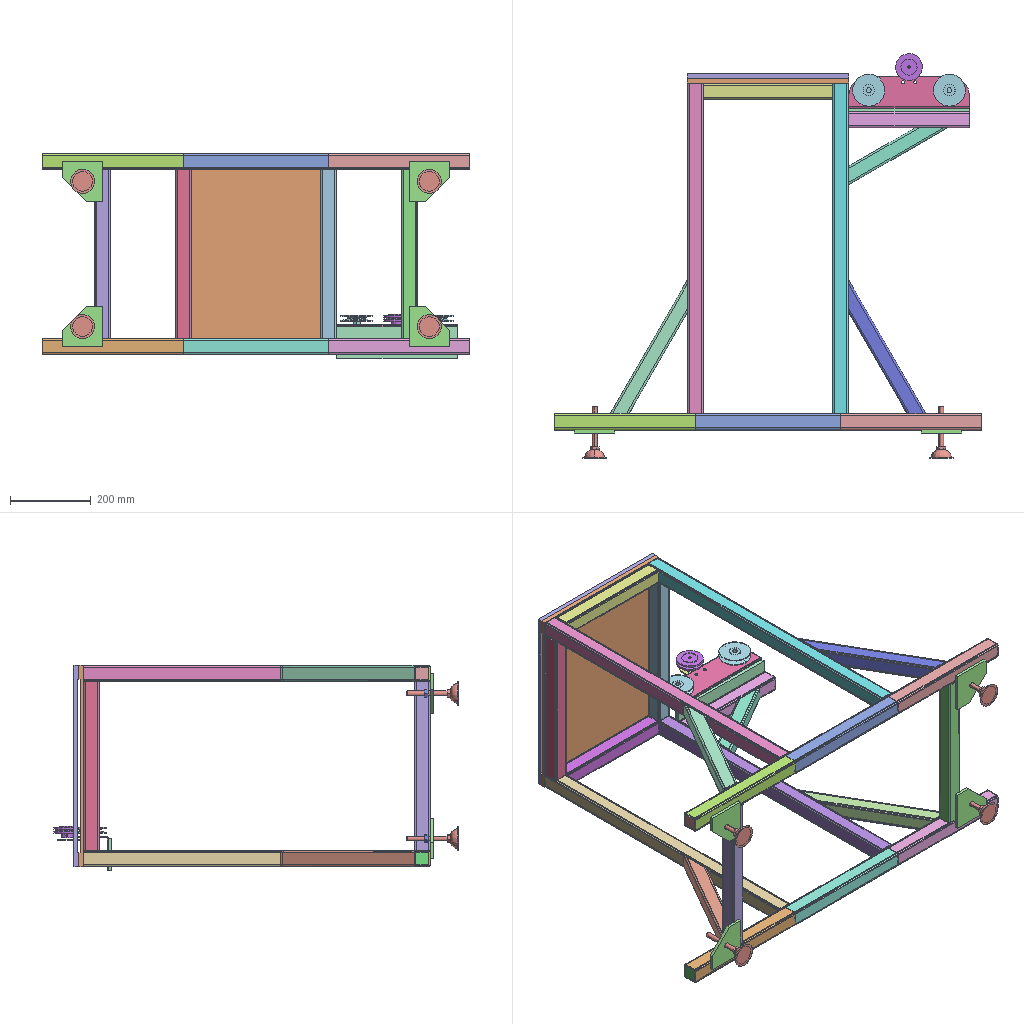Assembly | SolidWorks | 12 different items | 19 placed | box 1060 x 1004 x 510 mm
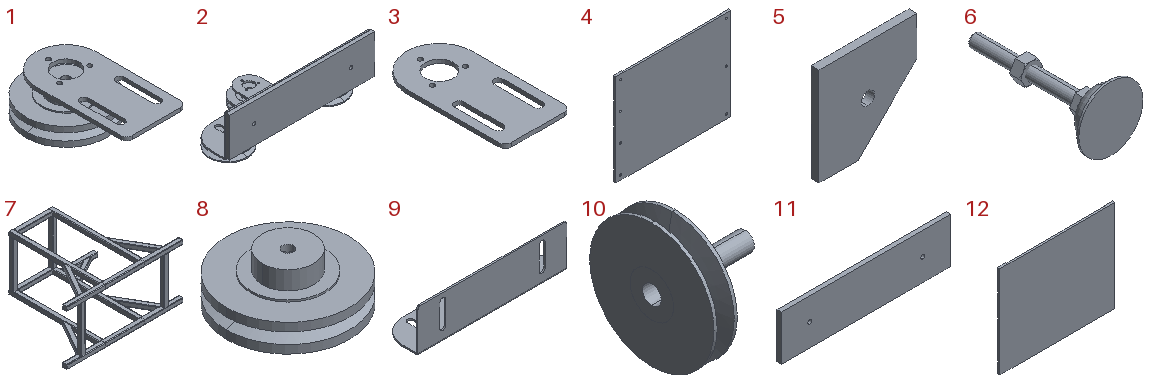Parts list (item | name | quantity | parent item | size | volume | features):
1 | (subassembly) | x1 | in 2 | 67 x 108.5 x 34.5 mm | 68724 mm3 | -
2 | (subassembly) | x1 | - | 300 x 143.899 x 110 mm | 501738 mm3 | features CompositeCurve 2, AEMSimFeature 1, LocalLPattern 1, ReferencePattern 1
3 | - | x1 | in 1 | 50 x 100 x 3 mm | 11541 mm3 | features ICE 2, Fillet 1, FlatPattern 1, HoleWzd 1, SMBaseFlange 1, SheetMetal 1
4 | - | x1 | - | 500 x 11.75 x 400 mm | 1689259 mm3 | features ICE 4, HoleWzd 2, Extrusion 1, Fillet 1
5 | - | x4 | - | 100 x 8 x 100 mm | 64455 mm3 | features Extrusion 1, HoleWzd 1
6 | - | x4 | - | 60 x 128 x 60 mm | 47779 mm3 | features ICE 4, Chamfer 1, Revolution 1
7 | - | x1 | - | 1060 x 860 x 500 mm | 4110495 mm3 | features 3DProfileFeature 1, EndCap 1, WeldCornerFeat 1, WeldMemberFeat 1, WeldmentFeature 1
8 | - | x1 | in 1 | 67 x 67 x 28 mm | 57183 mm3 | features ICE 4, 3DProfileFeature 1, Extrusion 1, HoleWzd 1, RevCut 1
9 | - | x1 | in 2 | 300 x 80 x 85 mm | 135508 mm3 | features Fillet 2, ICE 2, EdgeFlange 1, FlatPattern 1, HoleWzd 1, SMBaseFlange 1, SheetMetal 1
10 | - | x2 | in 2 | 60 x 80 x 80 mm | 53043 mm3 | features ICE 5, Revolution 1
11 | - | x1 | in 2 | 300 x 8 x 80 mm | 191419 mm3 | features Extrusion 1, HoleWzd 1
12 | - | x1 | - | 500 x 11.75 x 400 mm | 1696904 mm3 | features ICE 4, Extrusion 1, Fillet 1
Mates (type | each side: item.copy, entity, surface, feature):
In the top assembly
Coincident | 7.1 face plane Cold-formed square hollow section 40×3(2) | 4.1 face plane Boss-Extrude1 | 3 times
Coincident | 4.1 face plane Cut-Extrude2 | 12.1 face plane Cut-Extrude2
Coincident | 4.1 face plane Boss-Extrude1 | 12.1 face plane Boss-Extrude1 | 2 times
Coincident | 7.1 face plane Cold-formed square hollow section 40×3(2) | 5.1 face plane Boss-Extrude1
DistanceDim | 5.1 face plane Boss-Extrude1 | 7.1 face plane Cold-formed square hollow section 40×3(2) | 2 times
DistanceDim | 5.2 face plane Boss-Extrude1 | 7.1 face plane Cold-formed square hollow section 40×3(2)
Coincident | 5.1 face plane Boss-Extrude1 | 5.2 face plane Boss-Extrude1 | 2 times
DistanceDim | 5.3 face plane Boss-Extrude1 | 7.1 face plane Cold-formed square hollow section 40×3(2) | 2 times
Coincident | 5.1 face plane Boss-Extrude1 | 5.3 face plane Boss-Extrude1
DistanceDim | 5.4 face plane Boss-Extrude1 | 7.1 face plane Cold-formed square hollow section 40×3(2)
Coincident | 5.3 face plane Boss-Extrude1 | 5.4 face plane Boss-Extrude1 | 2 times
Coincident | 7.1 face plane Cold-formed square hollow section 40×3(2) | 11.1 face plane Boss-Extrude1 | 2 times
DistanceDim | 11.1 face plane Boss-Extrude1 | 7.1 face plane Cold-formed square hollow section 40×3(2)
Concentric | 5.2 face cylinder M12 Clearance Hole1 | 6.1 face cylinder Revolve1
Concentric | 5.1 face cylinder M12 Clearance Hole1 | 6.2 face cylinder Revolve1
Concentric | 5.4 face cylinder M12 Clearance Hole1 | 6.3 face cylinder Revolve1
Concentric | 5.3 face cylinder M12 Clearance Hole1 | 6.4 face cylinder Revolve1
Coincident | 6.3 face plane Revolve1 | 6.4 face plane Revolve1
Coincident | 6.1 face plane Revolve1 | 6.3 face plane Revolve1
Coincident | 6.1 face plane Revolve1 | 6.2 face plane Revolve1
In subassembly 2
Coincident | 9.1 face plane Base-Flange1 | 10.1 face plane Boss-Extrude2
Parallel | 9.1 face plane Edge-Flange1 | 10.1 plane
Concentric | 9.1 edge | 10.1 face cylinder Boss-Extrude2
Parallel | 9.1 face plane Base-Flange1 | 3.1 face plane Base-Flange1
Coincident | 9.1 face plane Edge-Flange1 | 11.2 face plane Boss-Extrude1 | 3 times